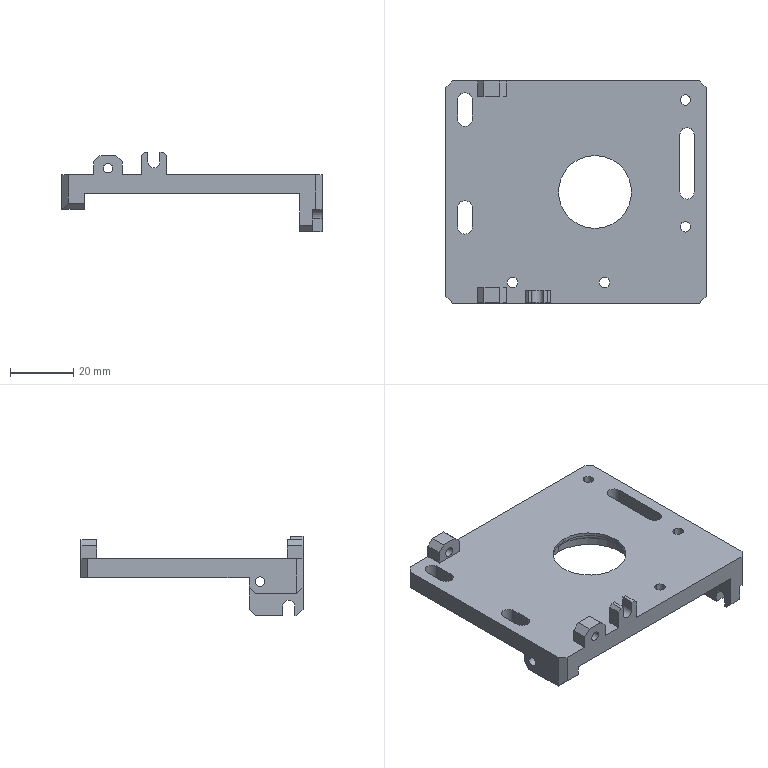NC program | NX | posted with a generic post | part box 82 x 70 x 25 mm
Lines 7084 to 7981 of 7981:
(FIXED_CONTOUR , TOOL : R1)
N14130 T02 M6
N14132 G54
N14134 G17 G0 G90 X-21.364 Y36. S9500 M3
N14136 G43 Z30. H2
N14138 Z1.2
N14140 G94 G1 Z-2.222 F2800.
N14142 Y35.966 Z-2.481
N14144 Y35.866 Z-2.722
N14146 Y35.707 Z-2.929
N14148 Y35.5 Z-3.088
N14150 Y35.259 Z-3.188
N14152 Y35. Z-3.222
N14154 Y30.
N14156 X-21.434 Z-3.152
N14158 Y35.
N14160 X-21.505 Z-3.081
N14162 Y30.
N14164 X-21.576 Z-3.01
N14166 Y35.
N14168 X-21.646 Z-2.94
N14170 Y30.
N14172 X-21.717 Z-2.869
N14174 Y35.
N14176 X-21.788 Z-2.798
N14178 Y30.
N14180 X-21.858 Z-2.727
N14182 Y35.
N14184 X-21.929 Z-2.657
N14186 Y30.
N14188 X-22. Z-2.586
N14190 Y35.
N14192 X-22.07 Z-2.515
N14194 Y30.
N14196 X-22.141 Z-2.445
N14198 Y35.
N14200 X-22.212 Z-2.374
N14202 Y30.
N14204 X-22.282 Z-2.303
N14206 Y35.
N14208 X-22.353 Z-2.233
N14210 Y30.
N14212 X-22.424 Z-2.162
N14214 Y35.
N14216 X-22.495 Z-2.091
N14218 X-22.494 Y30.
N14220 X-22.565 Z-2.021
N14222 Y35.
N14224 X-22.636 Z-1.95
N14226 Y30.
N14228 X-22.707 Z-1.879
N14230 Y35.
N14232 X-22.777 Z-1.809
N14234 Y30.
N14236 X-22.848 Z-1.738
N14238 Y35.
N14240 X-22.919 Z-1.667
N14242 Y30.
N14244 X-22.989 Z-1.597
N14246 Y35.
N14248 X-23.06 Z-1.526
N14250 Y30.
N14252 X-23.131 Z-1.455
N14254 Y35.
N14256 X-23.201 Z-1.385
N14258 Y30. Z-1.384
N14260 X-23.272 Z-1.314
N14262 Y35.
N14264 Y35.259 Z-1.28
N14266 Y35.5 Z-1.18
N14268 Y35.707 Z-1.021
N14270 Y35.866 Z-0.814
N14272 Y35.966 Z-0.573
N14274 Y36. Z-0.314
N14276 Z2.
N14278 G0 Z30.
N14280 X-31.636 Y29.
N14282 Z1.2
N14284 G1 Z-2.222
N14286 Y29.034 Z-2.481
N14288 Y29.134 Z-2.722
N14290 Y29.293 Z-2.929
N14292 Y29.5 Z-3.088
N14294 Y29.741 Z-3.188
N14296 Y30. Z-3.222
N14298 Y35.
N14300 X-31.566 Z-3.152
N14302 Y30.
N14304 X-31.495 Z-3.081
N14306 Y35.
N14308 X-31.424 Z-3.01
N14310 Y30.
N14312 X-31.354 Z-2.94
N14314 Y35.
N14316 X-31.283 Z-2.869
N14318 Y30.
N14320 X-31.212 Z-2.798
N14322 Y35.
N14324 X-31.142 Z-2.727
N14326 Y30.
N14328 X-31.071 Z-2.657
N14330 Y35.
N14332 X-31. Z-2.586
N14334 Y30.
N14336 X-30.93 Z-2.515
N14338 Y35.
N14340 X-30.859 Z-2.445
N14342 Y30.
N14344 X-30.788 Z-2.374
N14346 Y35.
N14348 X-30.718 Z-2.303
N14350 Y30.
N14352 X-30.647 Z-2.233
N14354 Y35.
N14356 X-30.576 Z-2.162
N14358 Y30.
N14360 X-30.506 Z-2.091
N14362 X-30.505 Y35.
N14364 X-30.435 Z-2.021
N14366 Y30.
N14368 X-30.364 Z-1.95
N14370 Y35.
N14372 X-30.293 Z-1.879
N14374 Y30.
N14376 X-30.223 Z-1.809
N14378 Y35.
N14380 X-30.152 Z-1.738
N14382 Y30.
N14384 X-30.081 Z-1.667
N14386 Y35.
N14388 X-30.011 Z-1.597
N14390 Y30.
N14392 X-29.94 Z-1.526
N14394 Y35.
N14396 X-29.869 Z-1.455
N14398 Y30.
N14400 X-29.799 Z-1.384
N14402 Y35. Z-1.385
N14404 X-29.728 Z-1.314
N14406 Y30.
N14408 Y29.741 Z-1.28
N14410 Y29.5 Z-1.18
N14412 Y29.293 Z-1.021
N14414 Y29.134 Z-0.814
N14416 Y29.034 Z-0.573
N14418 Y29. Z-0.314
N14420 Z2.
N14422 G0 Z30.
N14424 X-31.636 Y-36.
N14426 Z1.2
N14428 G1 Z-2.222
N14430 Y-35.966 Z-2.481
N14432 Y-35.866 Z-2.722
N14434 Y-35.707 Z-2.929
N14436 Y-35.5 Z-3.088
N14438 Y-35.259 Z-3.188
N14440 Y-35. Z-3.222
N14442 Y-30.
N14444 X-31.566 Z-3.152
N14446 Y-35.
N14448 X-31.495 Z-3.081
N14450 Y-30.
N14452 X-31.424 Z-3.01
N14454 Y-35.
N14456 X-31.354 Z-2.94
N14458 Y-30.
N14460 X-31.283 Z-2.869
N14462 Y-35.
N14464 X-31.212 Z-2.798
N14466 Y-30.
N14468 X-31.142 Z-2.727
N14470 Y-35.
N14472 X-31.071 Z-2.657
N14474 Y-30.
N14476 X-31. Z-2.586
N14478 Y-35.
N14480 X-30.93 Z-2.515
N14482 Y-30.
N14484 X-30.859 Z-2.445
N14486 Y-35.
N14488 X-30.788 Z-2.374
N14490 Y-30.
N14492 X-30.718 Z-2.303
N14494 Y-35.
N14496 X-30.647 Z-2.233
N14498 Y-30.
N14500 X-30.576 Z-2.162
N14502 Y-35.
N14504 X-30.506 Z-2.091
N14506 X-30.505 Y-30.
N14508 X-30.435 Z-2.021
N14510 Y-35.
N14512 X-30.364 Z-1.95
N14514 Y-30.
N14516 X-30.293 Z-1.879
N14518 Y-35.
N14520 X-30.223 Z-1.809
N14522 Y-30.
N14524 X-30.152 Z-1.738
N14526 Y-35.
N14528 X-30.081 Z-1.667
N14530 Y-30.
N14532 X-30.011 Z-1.597
N14534 Y-35.
N14536 X-29.94 Z-1.526
N14538 Y-30.
N14540 X-29.869 Z-1.455
N14542 Y-35.
N14544 X-29.799 Z-1.384
N14546 Y-30. Z-1.385
N14548 X-29.728 Z-1.314
N14550 Y-35.
N14552 Y-35.259 Z-1.28
N14554 Y-35.5 Z-1.18
N14556 Y-35.707 Z-1.021
N14558 Y-35.866 Z-0.814
N14560 Y-35.966 Z-0.573
N14562 Y-36. Z-0.314
N14564 Z2.
N14566 G0 Z30.
N14568 X-21.364 Y-29.
N14570 Z1.2
N14572 G1 Z-2.222
N14574 Y-29.034 Z-2.481
N14576 Y-29.134 Z-2.722
N14578 Y-29.293 Z-2.929
N14580 Y-29.5 Z-3.088
N14582 Y-29.741 Z-3.188
N14584 Y-30. Z-3.222
N14586 Y-35.
N14588 X-21.434 Z-3.152
N14590 Y-30.
N14592 X-21.505 Z-3.081
N14594 Y-35.
N14596 X-21.576 Z-3.01
N14598 Y-30.
N14600 X-21.646 Z-2.94
N14602 Y-35.
N14604 X-21.717 Z-2.869
N14606 Y-30.
N14608 X-21.788 Z-2.798
N14610 Y-35.
N14612 X-21.858 Z-2.727
N14614 Y-30.
N14616 X-21.929 Z-2.657
N14618 Y-35.
N14620 X-22. Z-2.586
N14622 Y-30.
N14624 X-22.07 Z-2.515
N14626 Y-35.
N14628 X-22.141 Z-2.445
N14630 Y-30.
N14632 X-22.212 Z-2.374
N14634 Y-35.
N14636 X-22.282 Z-2.303
N14638 Y-30.
N14640 X-22.353 Z-2.233
N14642 Y-35.
N14644 X-22.424 Z-2.162
N14646 Y-30.
N14648 X-22.495 Z-2.091
N14650 X-22.494 Y-35.
N14652 X-22.565 Z-2.021
N14654 Y-30.
N14656 X-22.636 Z-1.95
N14658 Y-35.
N14660 X-22.707 Z-1.879
N14662 Y-30.
N14664 X-22.777 Z-1.809
N14666 Y-35.
N14668 X-22.848 Z-1.738
N14670 Y-30.
N14672 X-22.919 Z-1.667
N14674 Y-35.
N14676 X-22.989 Z-1.597
N14678 Y-30.
N14680 X-23.06 Z-1.526
N14682 Y-35.
N14684 X-23.131 Z-1.455
N14686 Y-30.
N14688 X-23.201 Z-1.385
N14690 Y-35. Z-1.384
N14692 X-23.272 Z-1.314
N14694 Y-30.
N14696 Y-29.741 Z-1.28
N14698 Y-29.5 Z-1.18
N14700 Y-29.293 Z-1.021
N14702 Y-29.134 Z-0.814
N14704 Y-29.034 Z-0.573
N14706 Y-29. Z-0.314
N14708 Z2.
N14710 G0 Z30.
N14712 X-15.777 Y-29.927
N14714 Z2.8
N14716 G1 Z0.557
N14718 Y-29.98 Z0.301
N14720 Y-30.098 Z0.068
N14722 Y-30.273 Z-0.126
N14724 Y-30.491 Z-0.269
N14726 Y-30.739 Z-0.35
N14728 Y-31. Z-0.364
N14730 Y-31.018 Z-0.363
N14732 Y-34.982
N14734 Y-35. Z-0.364
N14736 X-15.848 Z-0.434
N14738 Y-31.
N14740 X-15.918 Z-0.504
N14742 Y-35.
N14744 X-15.989 Z-0.575
N14746 Y-31.
N14748 X-16.06 Z-0.646
N14750 Y-35.
N14752 X-16.131 Z-0.716
N14754 X-16.13 Y-31.
N14756 X-16.201 Z-0.787
N14758 Y-35.
N14760 X-16.272 Z-0.858
N14762 Y-31.
N14764 X-16.343 Z-0.928
N14766 Y-35.
N14768 X-16.413 Z-0.999
N14770 Y-31.
N14772 X-16.484 Z-1.07
N14774 Y-35.
N14776 X-16.554 Z-1.141
N14778 Y-31.
N14780 X-16.625 Z-1.212
N14782 Y-31.017 Z-1.21
N14784 Y-34.983 Z-1.211
N14786 Y-35. Z-1.212
N14788 X-16.695 Z-1.283
N14790 Y-34.975 Z-1.281
N14792 Y-31.025
N14794 Y-31. Z-1.283
N14796 Y-30.739 Z-1.271
N14798 Y-30.491 Z-1.193
N14800 Y-30.27 Z-1.052
N14802 Y-30.094 Z-0.859
N14804 Y-29.974 Z-0.628
N14806 Y-29.918 Z-0.373
N14808 Z2.8
N14810 G0 Z30.
N14812 X-12.822 Y-36.381
N14814 Z2.8
N14816 G1 Z-3.839
N14818 X-12.83 Y-36.21 Z-4.036
N14820 X-12.841 Y-35.994 Z-4.182
N14822 X-12.853 Y-35.748 Z-4.268
N14824 X-12.866 Y-35.488 Z-4.287
N14826 X-12.879 Y-35.232 Z-4.238
N14828 X-12.89 Y-34.997 Z-4.124
N14830 X-12.892 Y-34.974 Z-4.106
N14832 X-12.897 Y-34.909 Z-4.031
N14834 X-12.898 Y-34.9 Z-4.011
N14836 X-12.9 Y-34.894 Z-3.975
N14838 Y-34.823 Z-1.125
N14840 Y-34.818 Z-1.1
N14842 Y-31.196
N14844 Y-31.165 Z-1.601
N14846 Y-31.107 Z-3.975
N14848 X-12.899 Y-31.104 Z-4.001
N14850 X-12.898 Y-31.101 Z-4.011
N14852 X-12.893 Y-31.034 Z-4.098
N14854 X-12.892 Y-31.026 Z-4.106
N14856 X-12.89 Y-31.003 Z-4.123
N14858 Y-31.031 Z-4.116
N14860 X-12.893 Y-31.16 Z-4.098
N14862 X-12.896 Y-31.195 Z-4.046
N14864 X-12.898 Y-31.203 Z-4.011
N14866 X-12.9 Y-31.207 Z-3.975
N14868 Y-31.242 Z-2.526
N14870 Y-31.28 Z-1.368
N14872 Y-31.293 Z-1.2
N14874 Y-34.718
N14876 Y-34.735 Z-1.622
N14878 X-12.899 Y-34.795 Z-3.998
N14880 X-12.898 Y-34.8 Z-4.021
N14882 X-12.895 Y-34.813 Z-4.061
N14884 X-12.893 Y-34.835 Z-4.098
N14886 X-12.89 Y-34.863 Z-4.117
N14888 Y-34.974
N14890 Y-34.997 Z-4.124
N14892 Y-34.974 Z-4.117
N14894 Y-34.863
N14896 X-12.893 Y-34.721 Z-4.101
N14898 X-12.898 Y-34.696 Z-4.011
N14900 X-12.9 Y-34.694 Z-3.975
N14902 Y-34.635 Z-1.604
N14904 Y-34.625 Z-1.38
N14906 Y-34.6 Z-1.3
N14908 Y-31.435
N14910 Y-31.343 Z-2.494
N14912 Y-31.307 Z-3.976
N14914 X-12.898 Y-31.304 Z-4.013
N14916 X-12.894 Y-31.286 Z-4.088
N14918 X-12.893 Y-31.28 Z-4.098
N14920 X-12.89 Y-31.111 Z-4.116
N14922 Y-31.026
N14924 Y-31.003 Z-4.123
N14926 Y-31.026 Z-4.116
N14928 Y-31.308
N14930 X-12.893 Y-31.386 Z-4.098
N14932 X-12.898 Y-31.404 Z-4.011
N14934 X-12.9 Y-31.407 Z-3.975
N14936 Y-31.441 Z-2.569
N14938 Y-31.489 Z-1.9
N14940 Y-31.552 Z-1.4
N14942 Y-34.501
N14944 Y-34.535 Z-1.625
N14946 X-12.899 Y-34.595 Z-3.988
N14948 X-12.897 Y-34.6 Z-4.04
N14950 X-12.891 Y-34.619 Z-4.11
N14952 X-12.89 Y-34.692 Z-4.117
N14954 Y-34.974
N14956 Y-34.997 Z-4.124
N14958 Y-34.974 Z-4.117
N14960 Y-34.58
N14962 X-12.892 Y-34.514 Z-4.104
N14964 X-12.895 Y-34.504 Z-4.069
N14966 X-12.898 Y-34.496 Z-4.011
N14968 X-12.9 Y-34.494 Z-3.975
N14970 Y-34.445 Z-2.006
N14972 Y-34.431 Z-1.605
N14974 Y-34.41 Z-1.5
N14976 Y-31.649
N14978 Y-31.59 Z-1.899
N14980 Y-31.537 Z-2.746
N14982 X-12.899 Y-31.506 Z-3.986
N14984 X-12.897 Y-31.501 Z-4.039
N14986 X-12.893 Y-31.489 Z-4.098
N14988 X-12.89 Y-31.357 Z-4.116
N14990 Y-31.026
N14992 Y-31.003 Z-4.123
N14994 Y-31.026 Z-4.116
N14996 Y-31.484
N14998 X-12.892 Y-31.59 Z-4.102
N15000 X-12.898 Y-31.605 Z-4.011
N15002 X-12.9 Y-31.607 Z-3.975
N15004 Y-31.639 Z-2.724
N15006 Y-31.68 Z-2.062
N15008 Y-31.735 Z-1.603
N15010 Y-31.815 Z-1.6
N15012 Y-34.325
N15014 Y-34.337 Z-1.772
N15016 Y-34.346 Z-2.059
N15018 Y-34.394 Z-3.975
N15020 X-12.898 Y-34.396 Z-4.015
N15022 X-12.892 Y-34.41 Z-4.102
N15024 X-12.89 Y-34.58 Z-4.117
N15026 Y-34.974
N15028 Y-34.997 Z-4.125
N15030 Y-34.974 Z-4.117
N15032 Y-34.315
N15034 Y-34.31 Z-4.115
N15036 X-12.898 Y-34.296 Z-4.014
N15038 X-12.9 Y-34.294 Z-3.975
N15040 Y-34.256 Z-2.436
N15042 Y-34.234 Z-1.736
N15044 Y-34.222 Z-1.7
N15046 Y-31.832
N15048 Y-31.81 Z-1.821
N15050 Y-31.787 Z-2.013
N15052 Y-31.773 Z-2.182
N15054 Y-31.739 Z-2.723
N15056 Y-31.707 Z-3.975
N15058 X-12.898 Y-31.705 Z-4.011
N15060 X-12.893 Y-31.692 Z-4.098
N15062 X-12.89 Y-31.59 Z-4.116
N15064 Y-31.026
N15066 Y-31.003 Z-4.124
N15068 Y-31.026 Z-4.116
N15070 Y-31.653
N15072 X-12.893 Y-31.793 Z-4.098
N15074 X-12.898 Y-31.805 Z-4.011
N15076 X-12.9 Y-31.807 Z-3.975
N15078 Y-31.833 Z-2.954
N15080 Y-31.872 Z-2.196
N15082 Y-31.924 Z-1.8
N15084 Y-34.128
N15086 Y-34.169 Z-2.981
N15088 Y-34.194 Z-3.975
N15090 X-12.897 Y-34.196 Z-4.025
N15092 X-12.892 Y-34.208 Z-4.105
N15094 X-12.89 Y-34.297 Z-4.117
N15096 Y-34.974
N15098 Y-34.997 Z-4.125
N15100 Y-34.974 Z-4.117
N15102 Y-34.128
N15104 X-12.892 Y-34.106 Z-4.102
N15106 X-12.898 Y-34.096 Z-4.021
N15108 X-12.9 Y-34.094 Z-3.975
N15110 Y-34.049 Z-2.408
N15112 Y-34.03 Z-1.9
N15114 Y-32.035
N15116 Y-32. Z-1.992
N15118 Y-31.966 Z-2.326
N15120 Y-31.92 Z-3.473
N15122 Y-31.907 Z-3.975
N15124 X-12.898 Y-31.905 Z-4.011
N15126 X-12.893 Y-31.895 Z-4.098
N15128 X-12.89 Y-31.872 Z-4.116
N15130 Y-31.026
N15132 Y-31.003 Z-4.124
N15134 Y-31.026 Z-4.116
N15136 Y-31.886 Z-4.117
N15138 X-12.893 Y-31.996 Z-4.098
N15140 X-12.898 Y-32.005 Z-4.011
N15142 X-12.9 Y-32.007 Z-3.975
N15144 Y-32.012 Z-3.777
N15146 Y-32.055 Z-2.583
N15148 Y-32.087 Z-2.121
N15150 Y-32.11 Z-2.
N15152 Y-33.928
N15154 Y-33.937 Z-2.058
N15156 Y-33.976 Z-3.346
N15158 Y-33.994 Z-3.975
N15160 X-12.896 Y-33.999 Z-4.051
N15162 X-12.893 Y-34.005 Z-4.1
N15164 X-12.89 Y-34.015 Z-4.117
N15166 Y-34.974
N15168 Y-34.997 Z-4.125
N15170 Y-34.974 Z-4.117
N15172 Y-34.014
N15174 X-12.892 Y-33.905 Z-4.105
N15176 X-12.899 Y-33.895 Z-4.005
N15178 X-12.9 Y-33.894 Z-3.975
N15180 Y-33.846 Z-2.345
N15182 Y-33.832 Z-2.1
N15184 Y-32.199
N15186 Y-32.154 Z-2.617
N15188 Y-32.117 Z-3.624
N15190 Y-32.107 Z-3.975
N15192 X-12.897 Y-32.104 Z-4.027
N15194 X-12.893 Y-32.096 Z-4.098
N15196 X-12.89 Y-31.947 Z-4.117
N15198 Y-31.026 Z-4.116
N15200 Y-31.003 Z-4.124
N15202 Y-31.026 Z-4.116
N15204 Y-32.154 Z-4.117
N15206 X-12.893 Y-32.197 Z-4.098
N15208 X-12.898 Y-32.205 Z-4.011
N15210 X-12.9 Y-32.207 Z-3.975
N15212 Y-32.236 Z-3.116
N15214 Y-32.261 Z-2.536
N15216 Y-32.273 Z-2.405
N15218 Y-32.295 Z-2.2
N15220 Y-33.732
N15222 Y-33.755 Z-2.638
N15224 Y-33.794 Z-3.975
N15226 X-12.897 Y-33.796 Z-4.027
N15228 X-12.892 Y-33.804 Z-4.105
N15230 X-12.89 Y-33.846 Z-4.117
N15232 Y-34.974 Z-4.118
N15234 Y-34.997 Z-4.125
N15236 Y-34.974 Z-4.118
N15238 Y-33.732 Z-4.117
N15240 X-12.892 Y-33.703 Z-4.102
N15242 X-12.898 Y-33.696 Z-4.02
N15244 X-12.9 Y-33.694 Z-3.975
N15246 Y-33.663 Z-2.926
N15248 Y-33.64 Z-2.362
N15250 Y-33.624 Z-2.3
N15252 Y-32.386
N15254 Y-32.371 Z-2.433
N15256 Y-32.358 Z-2.621
N15258 Y-32.339 Z-3.041
N15260 Y-32.307 Z-3.975
N15262 X-12.896 Y-32.302 Z-4.053
N15264 X-12.893 Y-32.298 Z-4.098
N15266 X-12.89 Y-32.18 Z-4.117
N15268 Y-31.026
N15270 Y-31.003 Z-4.124
N15272 Y-31.026 Z-4.117
N15274 Y-32.241
N15276 X-12.893 Y-32.398 Z-4.098
N15278 X-12.898 Y-32.406 Z-4.011
N15280 X-12.9 Y-32.407 Z-3.975
N15282 Y-32.436 Z-3.125
N15284 Y-32.473 Z-2.413
N15286 Y-32.511 Z-2.4
N15288 Y-33.532
N15290 Y-33.543 Z-2.425
N15292 Y-33.564 Z-2.947
N15294 Y-33.594 Z-3.975
N15296 X-12.898 Y-33.596 Z-4.022
N15298 X-12.892 Y-33.603 Z-4.103
N15300 X-12.89 Y-33.731 Z-4.117
N15302 Y-34.974 Z-4.118
N15304 Y-34.997 Z-4.125
N15306 Y-34.974 Z-4.118
N15308 Y-33.564 Z-4.117
N15310 X-12.891 Y-33.503 Z-4.108
N15312 X-12.898 Y-33.495 Z-4.011
N15314 X-12.9 Y-33.494 Z-3.975
N15316 Y-33.462 Z-2.905
N15318 Y-33.445 Z-2.5
N15320 Y-32.576
N15322 Y-32.565 Z-2.574
N15324 Y-32.525 Z-3.449
N15326 Y-32.507 Z-3.975
N15328 X-12.893 Y-32.498 Z-4.098
N15330 X-12.89 Y-32.436 Z-4.117
N15332 Y-31.026
N15334 Y-31.003 Z-4.124
N15336 Y-31.026 Z-4.117
N15338 Y-32.473
N15340 X-12.893 Y-32.599 Z-4.098
N15342 X-12.9 Y-32.607 Z-3.975
N15344 Y-32.635 Z-3.213
N15346 Y-32.663 Z-2.618
N15348 Y-32.669 Z-2.6
N15350 Y-33.347
N15352 Y-33.367 Z-3.075
N15354 X-12.899 Y-33.394 Z-3.997
N15356 X-12.892 Y-33.402 Z-4.104
N15358 X-12.89 Y-33.449 Z-4.117
N15360 Y-34.974 Z-4.118
N15362 Y-34.997 Z-4.126
N15364 Y-34.974 Z-4.118
N15366 Y-33.448
N15368 X-12.893 Y-33.301 Z-4.1
N15370 X-12.9 Y-33.294 Z-3.975
N15372 Y-33.268 Z-3.157
N15374 Y-33.253 Z-2.741
N15376 Y-33.244 Z-2.7
N15378 Y-32.778
N15380 Y-32.737 Z-3.186
N15382 Y-32.707 Z-3.977
N15384 X-12.893 Y-32.699 Z-4.098
N15386 X-12.89 Y-32.533 Z-4.117
N15388 Y-31.026
N15390 Y-31.003 Z-4.124
N15392 Y-31.026 Z-4.117
N15394 Y-32.718
N15396 X-12.893 Y-32.799 Z-4.098
N15398 X-12.9 Y-32.807 Z-3.975
N15400 Y-32.827 Z-3.446
N15402 Y-32.863 Z-2.887
N15404 Y-32.878 Z-2.8
N15406 Y-33.154
N15408 Y-33.186 Z-3.711
N15410 Y-33.194 Z-3.975
N15412 X-12.891 Y-33.202 Z-4.112
N15414 X-12.89 Y-33.282 Z-4.118
N15416 Y-34.974
N15418 Y-34.997 Z-4.126
N15420 Y-34.974 Z-4.118
N15422 Y-33.166
N15424 X-12.892 Y-33.101 Z-4.105
N15426 X-12.9 Y-33.094 Z-3.975
N15428 Y-33.07 Z-3.237
N15430 Y-33.051 Z-2.9
N15432 Y-32.965
N15434 Y-32.959 Z-2.943
N15436 Y-32.93 Z-3.391
N15438 Y-32.907 Z-3.975
N15440 X-12.893 Y-32.9 Z-4.098
N15442 X-12.89 Y-32.766 Z-4.118
N15444 Y-31.026 Z-4.117
N15446 Y-31.003 Z-4.125
N15448 Y-31.026 Z-4.117
N15450 Y-32.766 Z-4.118
N15452 X-12.893 Y-32.9 Z-4.098
N15454 Y-33.1
N15456 X-12.892 Y-33.101 Z-4.105
N15458 X-12.89 Y-33.166 Z-4.118
N15460 Y-34.974
N15462 Y-34.997 Z-4.126
N15464 X-12.885 Y-34.998 Z-4.154
N15466 X-12.871 Z-4.2
N15468 Y-34.974 Z-4.195
N15470 Y-31.026
N15472 Y-31.002 Z-4.199
N15474 X-12.842 Y-31.001 Z-4.295
N15476 Y-31.026 Z-4.291
N15478 Y-34.974
N15480 Y-35. Z-4.295
N15482 X-12.802 Z-4.387
N15484 Y-34.974 Z-4.382
N15486 X-12.803 Y-31.026
N15488 Y-31. Z-4.386
N15490 X-12.792 Z-4.411
N15492 X-12.756 Z-4.474
N15494 Y-31.026 Z-4.471
N15496 Y-34.974
N15498 Y-35. Z-4.474
N15500 X-12.733 Z-4.512
N15502 X-12.699 Z-4.553
N15504 Y-31.
N15506 X-12.674 Z-4.583
N15508 X-12.63 Z-4.626
N15510 Y-35. Z-4.625
N15512 X-12.558 Z-4.693
N15514 Y-31.023 Z-4.692
N15516 Y-31. Z-4.695
N15518 X-12.54 Z-4.711
N15520 X-12.476 Z-4.75
N15522 Y-35.
N15524 X-12.39 Z-4.802
N15526 Y-34.974 Z-4.8
N15528 Y-31.026
N15530 Y-31. Z-4.802
N15532 X-12.298 Z-4.839
N15534 Y-31.026 Z-4.838
N15536 Y-34.98
N15538 Y-35. Z-4.839
N15540 X-12.269 Z-4.851
N15542 X-12.202 Z-4.869
N15544 X-12.203 Y-31.
N15546 X-12.135 Z-4.888
N15548 X-12.105 Z-4.89
N15550 Y-35.
N15552 X-12.005 Z-4.899
N15554 Y-31.
N15556 X-11.977 Z-4.898
N15558 X-11.906 Z-4.891
N15560 X-11.905 Y-35.
N15562 X-11.861 Z-4.886
N15564 X-11.807 Z-4.872
N15566 X-11.808 Y-31.
N15568 X-11.722 Z-4.847
N15570 X-11.712 Z-4.843
N15572 Y-31.026 Z-4.842
N15574 Y-34.974
N15576 Y-35. Z-4.843
N15578 X-11.619 Z-4.805
N15580 Y-34.974 Z-4.804
N15582 X-11.62 Y-31.026
N15584 Y-31. Z-4.806
N15586 X-11.583 Z-4.786
N15588 X-11.533 Z-4.756
N15590 Y-35.
N15592 X-11.46 Z-4.712
N15594 X-11.449 Z-4.702
N15596 Y-34.976 Z-4.699
N15598 X-11.45 Y-31.024
N15600 Y-31. Z-4.702
N15602 X-11.378 Z-4.633
N15604 Y-31.01 Z-4.631
N15606 X-11.377 Y-35. Z-4.632
N15608 X-11.325 Z-4.582
N15610 X-11.307 Z-4.561
N15612 Y-31.
N15614 X-11.266 Z-4.512
N15616 X-11.249 Z-4.482
N15618 Y-31.026 Z-4.479
N15620 Y-34.974
N15622 Y-35. Z-4.482
N15624 X-11.208 Z-4.411
N15626 X-11.201 Z-4.395
N15628 Y-34.974 Z-4.391
N15630 X-11.202 Y-31.026
N15632 Y-31. Z-4.396
N15634 X-11.162 Y-31.001 Z-4.304
N15636 Y-31.026 Z-4.3
N15638 X-11.161 Y-34.974 Z-4.299
N15640 Y-34.999 Z-4.304
N15642 X-11.15 Z-4.271
N15644 X-11.131 Y-34.998 Z-4.208
N15646 Y-34.974 Z-4.204
N15648 X-11.132 Y-31.026
N15650 Y-31.002 Z-4.209
N15652 X-11.113 Y-31.003 Z-4.143
N15654 X-11.108 Z-4.115
N15656 Y-31.026 Z-4.108
N15658 Y-34.974 Z-4.107
N15660 Y-34.997 Z-4.114
N15662 X-11.101 Y-34.995 Z-4.009
N15664 X-11.102 Y-34.974 Z-4.007
N15666 Y-31.026 Z-4.008
N15668 X-11.101 Y-31.003 Z-4.011
N15670 X-11.099 Z-3.91
N15672 X-11.1 Y-31.025 Z-3.908
N15674 Y-34.977 Z-3.907
N15676 X-11.099 Y-34.992 Z-3.908
N15678 Y-34.99 Z-3.808
N15680 X-11.1 Y-31.024
N15682 X-11.099 Y-31.003 Z-3.81
N15684 Z-3.709
N15686 X-11.1 Y-31.024 Z-3.708
N15688 X-11.099 Y-34.987 Z-3.707
N15690 Y-34.985 Z-3.607
N15692 X-11.1 Y-31.02 Z-3.608
N15694 X-11.099 Y-31.003 Z-3.609
N15696 Z-3.509
N15698 X-11.1 Y-34.982 Z-3.507
N15700 Y-34.98 Z-3.407
N15702 X-11.099 Y-31.003 Z-3.409
N15704 Z-3.309
N15706 X-11.1 Y-34.977 Z-3.307
N15708 Y-34.975 Z-3.207
N15710 X-11.099 Y-31.003 Z-3.209
N15712 Y-31.002 Z-3.109
N15714 X-11.1 Y-34.973 Z-3.107
N15716 Y-34.97 Z-3.007
N15718 X-11.099 Y-31.002 Z-3.009
N15720 Z-2.909
N15722 X-11.1 Y-34.968 Z-2.907
N15724 Y-34.965 Z-2.807
N15726 X-11.099 Y-31.002 Z-2.809
N15728 Z-2.709
N15730 X-11.1 Y-34.963 Z-2.707
N15732 Y-34.96 Z-2.607
N15734 X-11.099 Y-31.002 Z-2.608
N15736 Z-2.508
N15738 X-11.1 Y-34.958 Z-2.507
N15740 Y-34.955 Z-2.407
N15742 X-11.099 Y-31.002 Z-2.408
N15744 Z-2.308
N15746 X-11.1 Y-34.953 Z-2.307
N15748 Y-34.95 Z-2.207
N15750 X-11.099 Y-31.002 Z-2.208
N15752 Z-2.108
N15754 X-11.1 Y-34.948 Z-2.107
N15756 Y-34.945 Z-2.007
N15758 X-11.099 Y-31.001 Z-2.008
N15760 Z-1.908
N15762 X-11.1 Y-34.943 Z-1.907
N15764 Y-34.94 Z-1.807
N15766 X-11.099 Y-31.001 Z-1.808
N15768 Z-1.708
N15770 X-11.1 Y-34.938 Z-1.707
N15772 Y-34.935 Z-1.607
N15774 X-11.099 Y-31.001 Z-1.608
N15776 Z-1.508
N15778 X-11.1 Y-34.933 Z-1.507
N15780 Y-34.93 Z-1.407
N15782 X-11.099 Y-31.001 Z-1.408
N15784 Z-1.308
N15786 X-11.1 Y-34.928 Z-1.307
N15788 Y-34.925 Z-1.207
N15790 X-11.099 Y-31.001 Z-1.208
N15792 Z-1.108
N15794 X-11.1 Y-34.923 Z-1.107
N15796 Y-34.92 Z-1.007
N15798 X-11.099 Y-31.001 Z-1.008
N15800 X-11.086 Y-30.742 Z-0.977
N15802 X-11.075 Y-30.5 Z-0.88
N15804 X-11.065 Y-30.291 Z-0.724
N15806 X-11.058 Y-30.13 Z-0.519
N15808 X-11.053 Y-30.027 Z-0.279
N15810 X-11.051 Y-29.99 Z-0.02
N15812 Z2.93
N15814 G0 Z3.73
N15816 X-7.364 Y-29.918
N15818 Z2.53
N15820 G1 Z-0.313
N15822 Y-29.974 Z-0.568
N15824 Y-30.094 Z-0.8
N15826 Y-30.271 Z-0.992
N15828 Y-30.491 Z-1.133
N15830 Y-30.739 Z-1.212
N15832 Y-31. Z-1.224
N15834 Y-31.018 Z-1.222
N15836 Y-34.982
N15838 Y-35. Z-1.224
N15840 X-7.434 Z-1.153
N15842 Y-31. Z-1.152
N15844 X-7.505 Z-1.081
N15846 Y-35.
N15848 X-7.575 Z-1.01
N15850 Y-31.
N15852 X-7.646 Z-0.94
N15854 Y-35.
N15856 X-7.717 Z-0.869
N15858 Y-31.
N15860 X-7.788 Z-0.798
N15862 X-7.787 Y-35.
N15864 X-7.858 Z-0.728
N15866 Y-31.
N15868 X-7.929 Z-0.657
N15870 Y-35.
N15872 X-8. Z-0.586
N15874 Y-31.
N15876 X-8.07 Z-0.516
N15878 Y-35.
N15880 X-8.141 Z-0.446
N15882 Y-31.
N15884 X-8.212 Z-0.376
N15886 Y-31.017 Z-0.374
N15888 Y-34.983
N15890 Y-35. Z-0.375
N15892 X-8.282 Z-0.305
N15894 Y-34.975 Z-0.303
N15896 Y-31.019 Z-0.304
N15898 Y-31. Z-0.307
N15900 Y-30.739 Z-0.314
N15902 Y-30.486 Z-0.253
N15904 Y-30.256 Z-0.128
N15906 Y-30.067 Z0.052
N15908 Y-29.931 Z0.274
N15910 Y-29.856 Z0.525
N15912 Z2.8
N15914 G0 Z30.
N15916 M5
N15918 M2